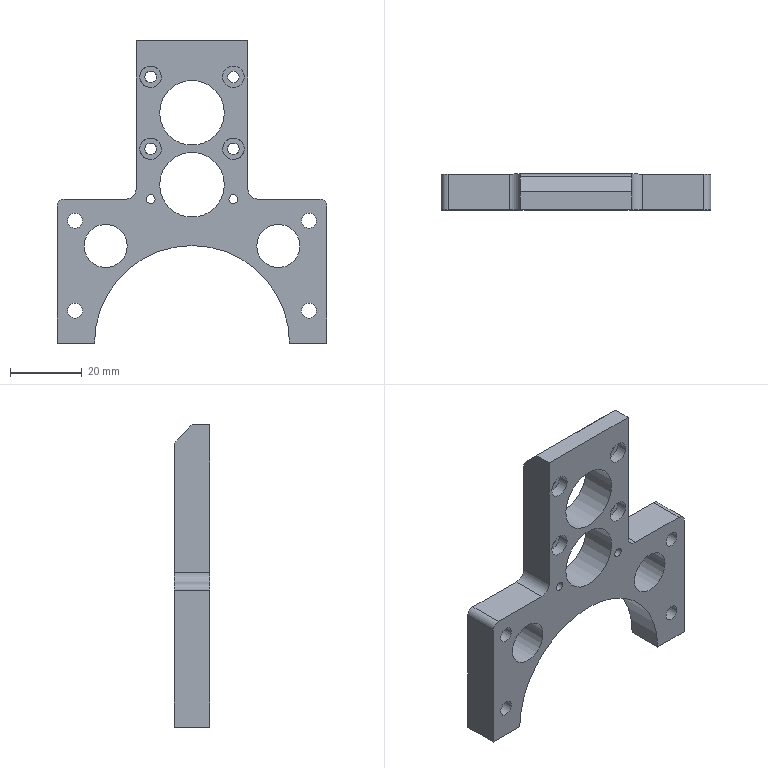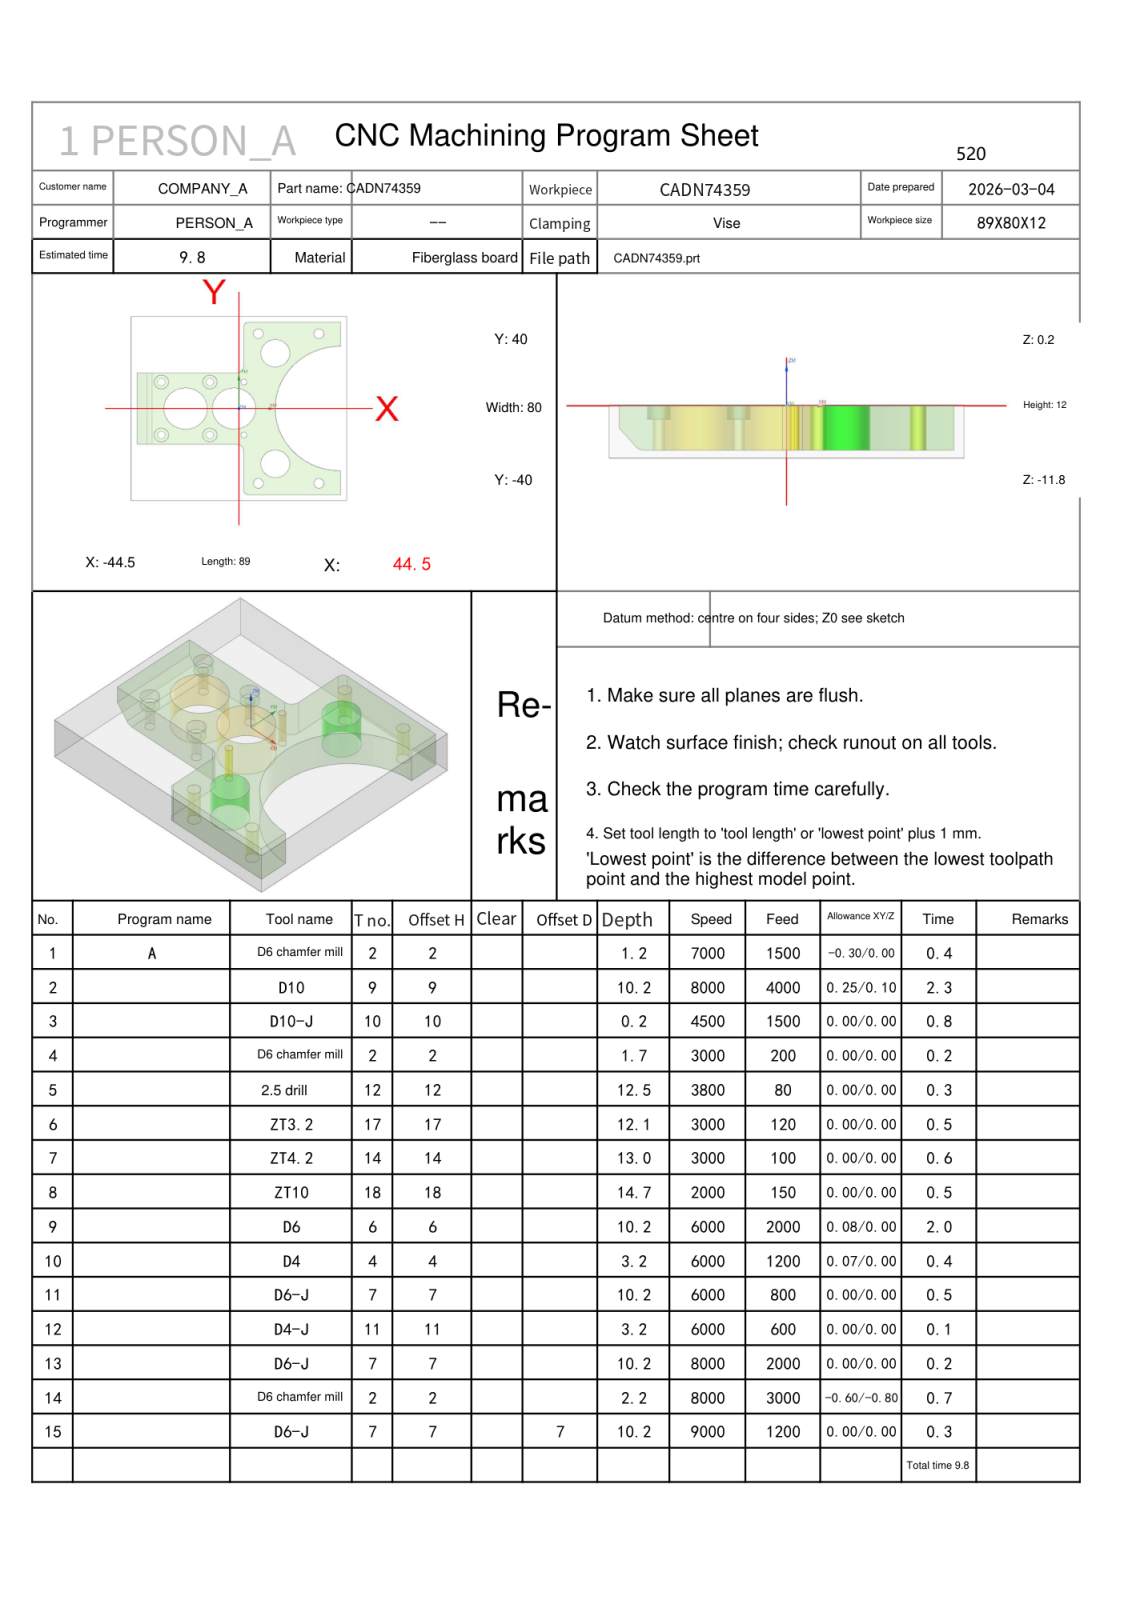NC program | NX | posted by the shop | part box 75 x 10 x 84 mm
Lines 1951 to 2989 of 4435:
N3 T10 M06
(D10-J  D=10. R=0. H=10 ce=0.00 di=0.00)
G00 G90 G54 X52. Y-35.962 M03 S4500
G43 H10 Z50.
M08
Z2.
G01 Z0.0 F1500.
X47.
X-47.
Y-29.423
X47.
Y-22.885
X-47.
Y-16.346
X47.
Y-9.808
X-47.
Y-3.269
X47.
Y3.269
X-47.
Y9.808
X47.
Y16.346
X-47.
Y22.885
X47.
Y29.423
X-47.
Y35.962
X47.
X52.
Z2.
G00 Z50.
G91 G28 Z0.0
M05
M09
G91 G28 Z0.0
M01
N4 T02 M06
(D6 chamfer mill  D=6. R=0. H=02 ce=0.00 di=0.00)
G00 G90 G54 X2. Y11.5 M03 S3000
G43 H02 Z50.
M08
G98 G81 X2. Y11.5 Z-1. R1. F200.
Y-11.5
G80
G00 Z50.
G00 G90 X33. Y-32.5 M03 S3000
Z50.
G98 G81 X33. Y-32.5 Z-1.5 R1. F200.
X15. Y-24.
X8. Y-32.5
X-12. Y-11.5
X-32.
X-22. Y0.0
X-32. Y11.5
X-12.
X-2. Y0.0
X8. Y32.5
X15. Y24.
X33. Y32.5
G80
G00 Z50.
G91 G28 Z0.0
M05
M09
G91 G28 Z0.0
M01
N5 T12 M06
(2.5 drill D=2.5 DR_a=118 H=12)
G00 G90 G54 X2. Y11.5 M03 S3800
G43 H12 Z50.
M08
G98 G83 X2. Y11.5 Z-12.251 R1. F80. Q1.5
Y-11.5
G80
G00 Z50.
G91 G28 Z0.0
M05
M09
G91 G28 Z0.0
M01
N6 T17 M06
(ZT3.2 D=3.2 DR_a=120 H=17)
G00 G90 G54 X-12. Y-11.5 M03 S3000
G43 H17 Z50.
M08
G98 G83 X-12. Y-11.5 Z-11.924 R1. F120. Q3.
X-32.
Y11.5
X-12.
G80
G00 Z50.
G91 G28 Z0.0
M05
M09
G91 G28 Z0.0
M01
N7 T14 M06
(ZT4.2 D=4.2 DR_a=118 H=14)
G00 G90 G54 X33. Y32.5 M03 S3000
G43 H14 Z50.
M08
G98 G83 X33. Y32.5 Z-12.762 R1. F100. Q1.5
X8.
Y-32.5
X33.
G80
G00 Z50.
G91 G28 Z0.0
M05
M09
G91 G28 Z0.0
M01
N8 T18 M06
(ZT10 D=10. DR_a=118 H=18)
G00 G90 G54 X15. Y-24. M03 S2000
G43 H18 Z50.
M08
G98 G83 X15. Y-24. Z-14.004 R1. F150. Q3.
Y24.
G80
G00 Z50.
G00 G90 X-22. Y0.0 M03 S2000
Z50.
G98 G83 X-22. Y0.0 Z-14.504 R1. F120. Q1.5
X-2.
G80
G00 Z50.
G91 G28 Z0.0
M05
M09
G91 G28 Z0.0
M01
N9 T06 M06
(D6  D=6. R=0. H=06 ce=0.10 di=0.00)
G00 G90 G54 X15. Y-24. M03 S6000
G43 H06 Z50.
M08
Z.3
G03 X16.45 Y-22.55 I0.0 J1.45 F2000.
X15. Y-21.1 I-1.45 J0.0
X15. Y-21.1 Z-.2 I0.0 J-2.9
X15. Y-21.1 Z-.7 I0.0 J-2.9
X15. Y-21.1 Z-1.2 I0.0 J-2.9
X15. Y-21.1 Z-1.7 I0.0 J-2.9
X15. Y-21.1 Z-2.2 I0.0 J-2.9
X15. Y-21.1 Z-2.7 I0.0 J-2.9
X15. Y-21.1 Z-3.2 I0.0 J-2.9
X15. Y-21.1 Z-3.7 I0.0 J-2.9
X15. Y-21.1 Z-4.2 I0.0 J-2.9
X15. Y-21.1 Z-4.7 I0.0 J-2.9
X15. Y-21.1 Z-5.2 I0.0 J-2.9
X15. Y-21.1 Z-5.7 I0.0 J-2.9
X15. Y-21.1 Z-6.2 I0.0 J-2.9
X15. Y-21.1 Z-6.7 I0.0 J-2.9
X15. Y-21.1 Z-7.2 I0.0 J-2.9
X15. Y-21.1 Z-7.7 I0.0 J-2.9
X15. Y-21.1 Z-8.2 I0.0 J-2.9
X15. Y-21.1 Z-8.7 I0.0 J-2.9
X15. Y-21.1 Z-9.2 I0.0 J-2.9
X15. Y-21.1 Z-9.7 I0.0 J-2.9
X16.705 Y-26.346 Z-10. I0.0 J-2.9
X17.9 Y-24. I-1.705 J2.346
X15. Y-21.1 I-2.9 J0.0
X12.1 Y-24. I0.0 J-2.9
X15. Y-26.9 I2.9 J0.0
X16.705 Y-26.346 I0.0 J2.9
X17.302 Y-25.173 I-.852 J1.173
X15.852 Y-23.723 I-1.45 J0.0
X15. Y-24. I0.0 J-1.45
G00 Z50.
Y24.
Z.3
G03 X16.45 Y25.45 I0.0 J1.45
X15. Y26.9 I-1.45 J0.0
X15. Y26.9 Z-.2 I0.0 J-2.9
X15. Y26.9 Z-.7 I0.0 J-2.9
X15. Y26.9 Z-1.2 I0.0 J-2.9
X15. Y26.9 Z-1.7 I0.0 J-2.9
X15. Y26.9 Z-2.2 I0.0 J-2.9
X15. Y26.9 Z-2.7 I0.0 J-2.9
X15. Y26.9 Z-3.2 I0.0 J-2.9
X15. Y26.9 Z-3.7 I0.0 J-2.9
X15. Y26.9 Z-4.2 I0.0 J-2.9
X15. Y26.9 Z-4.7 I0.0 J-2.9
X15. Y26.9 Z-5.2 I0.0 J-2.9
X15. Y26.9 Z-5.7 I0.0 J-2.9
X15. Y26.9 Z-6.2 I0.0 J-2.9
X15. Y26.9 Z-6.7 I0.0 J-2.9
X15. Y26.9 Z-7.2 I0.0 J-2.9
X15. Y26.9 Z-7.7 I0.0 J-2.9
X15. Y26.9 Z-8.2 I0.0 J-2.9
X15. Y26.9 Z-8.7 I0.0 J-2.9
X15. Y26.9 Z-9.2 I0.0 J-2.9
X15. Y26.9 Z-9.7 I0.0 J-2.9
X16.705 Y21.654 Z-10. I0.0 J-2.9
X17.9 Y24. I-1.705 J2.346
X15. Y26.9 I-2.9 J0.0
X12.1 Y24. I0.0 J-2.9
X15. Y21.1 I2.9 J0.0
X16.705 Y21.654 I0.0 J2.9
X17.302 Y22.827 I-.852 J1.173
X15.852 Y24.277 I-1.45 J0.0
X15. Y24. I0.0 J-1.45
G00 Z50.
G00 G90 X-22. Y0.0 M03 S6000
Z50.
Z.5
G03 X-20.75 Y1.25 I0.0 J1.25 F1800.
X-22. Y2.5 I-1.25 J0.0
X-22. Y2.5 Z.3 I0.0 J-2.5 F2000.
X-22. Y2.5 Z.1 I0.0 J-2.5
X-22. Y2.5 Z-.1 I0.0 J-2.5
X-22. Y2.5 Z-.3 I0.0 J-2.5
X-22. Y2.5 Z-.5 I0.0 J-2.5
X-22. Y2.5 Z-.7 I0.0 J-2.5
X-22. Y2.5 Z-.9 I0.0 J-2.5
X-22. Y2.5 Z-1.1 I0.0 J-2.5
X-22. Y2.5 Z-1.3 I0.0 J-2.5
X-22. Y2.5 Z-1.5 I0.0 J-2.5
X-22. Y2.5 Z-1.7 I0.0 J-2.5
X-22. Y2.5 Z-1.9 I0.0 J-2.5
X-22. Y2.5 Z-2.1 I0.0 J-2.5
X-22. Y2.5 Z-2.3 I0.0 J-2.5
X-22. Y2.5 Z-2.5 I0.0 J-2.5
X-22. Y2.5 Z-2.7 I0.0 J-2.5
X-22. Y2.5 Z-2.9 I0.0 J-2.5
X-22. Y2.5 Z-3.1 I0.0 J-2.5
X-22. Y2.5 Z-3.3 I0.0 J-2.5
X-22. Y2.5 Z-3.5 I0.0 J-2.5
X-22. Y2.5 Z-3.7 I0.0 J-2.5
X-22. Y2.5 Z-3.9 I0.0 J-2.5
X-22. Y2.5 Z-4.1 I0.0 J-2.5
X-22. Y2.5 Z-4.3 I0.0 J-2.5
X-22. Y2.5 Z-4.5 I0.0 J-2.5
X-22. Y2.5 Z-4.7 I0.0 J-2.5
X-24.5 Y0.0 Z-4.75 I0.0 J-2.5
X-21.984 Y-2.552 I2.552 J0.0
G01 X-21.947
G03 X-19.352 Y-.072 I0.0 J2.598
G01 X-19.35 Y.049
G03 X-21.868 Y2.72 I-2.675 J0.0
G01 X-22.03 Y2.724
G03 X-24.793 Y.153 I0.0 J-2.77
X-24.8 Y-.05 I2.817 J-.202
X-22.216 Y-2.863 I2.824 J0.0
X-21.968 Y-2.874 I.248 J2.908
X-19.064 Y-.241 I0.0 J2.919
X-19.049 Y.05 I-2.958 J.291
X-21.692 Y3.004 I-2.973 J0.0
X-22.033 Y3.023 I-.341 J-3.048
X-25.076 Y.338 I0.0 J-3.067
X-25.101 Y-.051 I3.097 J-.388
X-22.409 Y-3.142 I3.121 J0.0
X-21.966 Y-3.173 I.442 J3.186
X-18.787 Y-.442 I0.0 J3.216
X-18.749 Y.051 I-3.233 J.493
X-21.483 Y3.277 I-3.27 J0.0
X-22.035 Y3.323 I-.552 J-3.319
X-25.347 Y.554 I0.0 J-3.365
X-25.401 Y-.052 I3.365 J-.605
X-22.632 Y-3.408 I3.419 J0.0
X-21.964 Y-3.472 I.668 J3.449
X-18.524 Y-.673 I0.0 J3.514
X-18.449 Y.052 I-3.493 J.725
X-21.245 Y3.535 I-3.568 J0.0
X-22.037 Y3.622 I-.792 J-3.576
X-25.602 Y.8 I0.0 J-3.662
X-25.701 Y-.053 I3.617 J-.853
X-22.886 Y-3.658 I3.716 J0.0
X-21.962 Y-3.772 I.924 J3.697
X-18.277 Y-.934 I0.0 J3.811
X-18.149 Y.053 I-3.737 J.987
X-20.977 Y3.776 I-3.865 J0.0
X-22.039 Y3.921 I-1.063 J-3.814
X-25.839 Y1.076 I0.0 J-3.96
X-26.001 Y-.053 I3.852 J-1.129
X-23.168 Y-3.889 I4.014 J0.0
X-21.96 Y-4.071 I1.209 J3.927
X-18.05 Y-1.224 I0.0 J4.108
X-17.849 Y.054 I-3.961 J1.278
X-20.68 Y3.998 I-4.162 J0.0
X-22.041 Y4.221 I-1.361 J-4.034
X-26.056 Y1.379 I0.0 J-4.257
X-26.301 Y-.054 I4.066 J-1.433
X-23.479 Y-4.1 I4.311 J0.0
X-21.958 Y-4.371 I1.521 J4.135
X-17.844 Y-1.541 I0.0 J4.406
X-17.548 Y.054 I-4.165 J1.596
X-20.356 Y4.197 I-4.46 J0.0
X-22.043 Y4.521 I-1.687 J-4.231
X-26.251 Y1.71 I0.0 J-4.555
X-26.602 Y-.054 I4.257 J-1.764
X-23.815 Y-4.288 I4.608 J0.0
X-21.956 Y-4.671 I1.859 J4.32
X-17.661 Y-1.885 I0.0 J4.703
X-17.248 Y.055 I-4.344 J1.939
X-20.007 Y4.372 I-4.757 J0.0
X-22.045 Y4.821 I-2.037 J-4.403
X-26.42 Y2.065 I0.0 J-4.852
X-26.902 Y-.055 I4.424 J-2.12
X-24.176 Y-4.45 I4.906 J0.0
X-21.954 Y-4.97 I2.222 J4.48
X-17.505 Y-2.252 I0.0 J5.001
X-16.948 Y.055 I-4.498 J2.307
X-19.635 Y4.521 I-5.055 J0.0
X-22.047 Y5.12 I-2.412 J-4.55
X-26.563 Y2.444 I0.0 J-5.149
X-27.203 Y-.055 I4.564 J-2.499
X-24.56 Y-4.585 I5.203 J0.0
X-21.953 Y-5.27 I2.607 J4.612
X-17.376 Y-2.642 I0.0 J5.298
X-16.647 Y.055 I-4.623 J2.696
X-19.24 Y4.641 I-5.352 J0.0
X-22.048 Y5.42 I-2.808 J-4.667
X-26.677 Y2.844 I0.0 J-5.447
X-27.503 Y-.055 I4.675 J-2.899
X-24.964 Y-4.69 I5.501 J0.0
X-21.951 Y-5.57 I3.013 J4.715
X-17.278 Y-3.052 I0.0 J5.595
X-16.347 Y.055 I-4.719 J3.106
X-18.826 Y4.731 I-5.649 J0.0
X-22.049 Y5.72 I-3.223 J-4.755
X-26.76 Y3.263 I0.0 J-5.744
X-27.808 Y-.068 I4.774 J-3.332
X-25.344 Y-4.824 I5.822 J0.0
X-21.959 Y-5.899 I3.385 J4.794
X-17.211 Y-3.48 I0.0 J5.869
X-16.08 Y0.0 I-4.789 J3.48
X-22. Y5.92 I-5.92 J0.0
X-27.92 Y0.0 I0.0 J-5.92
X-22. Y-5.92 I5.92 J0.0
X-16.934 Y-3.063 I0.0 J5.92
X-16.507 Y-1.532 I-2.533 J1.532
X-19.467 Y1.428 I-2.96 J0.0
X-22. Y0.0 I0.0 J-2.96
X-20.75 Y1.25 I0.0 J1.25 F1800.
X-22. Y2.5 I-1.25 J0.0
X-22. Y2.5 Z-4.95 I0.0 J-2.5 F2000.
X-22. Y2.5 Z-5.15 I0.0 J-2.5
X-22. Y2.5 Z-5.35 I0.0 J-2.5
X-22. Y2.5 Z-5.55 I0.0 J-2.5
X-22. Y2.5 Z-5.75 I0.0 J-2.5
X-22. Y2.5 Z-5.95 I0.0 J-2.5
X-22. Y2.5 Z-6.15 I0.0 J-2.5
X-22. Y2.5 Z-6.35 I0.0 J-2.5
X-22. Y2.5 Z-6.55 I0.0 J-2.5
X-22. Y2.5 Z-6.75 I0.0 J-2.5
X-22. Y2.5 Z-6.95 I0.0 J-2.5
X-22. Y2.5 Z-7.15 I0.0 J-2.5
X-22. Y2.5 Z-7.35 I0.0 J-2.5
X-22. Y2.5 Z-7.55 I0.0 J-2.5
X-22. Y2.5 Z-7.75 I0.0 J-2.5
X-22. Y2.5 Z-7.95 I0.0 J-2.5
X-22. Y2.5 Z-8.15 I0.0 J-2.5
X-22. Y2.5 Z-8.35 I0.0 J-2.5
X-22. Y2.5 Z-8.55 I0.0 J-2.5
X-22. Y2.5 Z-8.75 I0.0 J-2.5
X-22. Y2.5 Z-8.95 I0.0 J-2.5
X-22. Y2.5 Z-9.15 I0.0 J-2.5
X-22. Y2.5 Z-9.35 I0.0 J-2.5
X-22. Y2.5 Z-9.55 I0.0 J-2.5
X-22. Y2.5 Z-9.75 I0.0 J-2.5
X-22. Y2.5 Z-9.95 I0.0 J-2.5
X-24.5 Y0.0 Z-10. I0.0 J-2.5
X-21.984 Y-2.552 I2.552 J0.0
G01 X-21.947
G03 X-19.352 Y-.072 I0.0 J2.598
G01 X-19.35 Y.049
G03 X-21.868 Y2.72 I-2.675 J0.0
G01 X-22.03 Y2.724
G03 X-24.793 Y.153 I0.0 J-2.77
X-24.8 Y-.05 I2.817 J-.202
X-22.216 Y-2.863 I2.824 J0.0
X-21.968 Y-2.874 I.248 J2.908
X-19.064 Y-.241 I0.0 J2.919
X-19.049 Y.05 I-2.958 J.291
X-21.692 Y3.004 I-2.973 J0.0
X-22.033 Y3.023 I-.341 J-3.048
X-25.076 Y.338 I0.0 J-3.067
X-25.101 Y-.051 I3.097 J-.388
X-22.409 Y-3.142 I3.121 J0.0
X-21.966 Y-3.173 I.442 J3.186
X-18.787 Y-.442 I0.0 J3.216
X-18.749 Y.051 I-3.233 J.493
X-21.483 Y3.277 I-3.27 J0.0
X-22.035 Y3.323 I-.552 J-3.319
X-25.347 Y.554 I0.0 J-3.365
X-25.401 Y-.052 I3.365 J-.605
X-22.632 Y-3.408 I3.419 J0.0
X-21.964 Y-3.472 I.668 J3.449
X-18.524 Y-.673 I0.0 J3.514
X-18.449 Y.052 I-3.493 J.725
X-21.245 Y3.535 I-3.568 J0.0
X-22.037 Y3.622 I-.792 J-3.576
X-25.602 Y.8 I0.0 J-3.662
X-25.701 Y-.053 I3.617 J-.853
X-22.886 Y-3.658 I3.716 J0.0
X-21.962 Y-3.772 I.924 J3.697
X-18.277 Y-.934 I0.0 J3.811
X-18.149 Y.053 I-3.737 J.987
X-20.977 Y3.776 I-3.865 J0.0
X-22.039 Y3.921 I-1.063 J-3.814
X-25.839 Y1.076 I0.0 J-3.96
X-26.001 Y-.053 I3.852 J-1.129
X-23.168 Y-3.889 I4.014 J0.0
X-21.96 Y-4.071 I1.209 J3.927
X-18.05 Y-1.224 I0.0 J4.108
X-17.849 Y.054 I-3.961 J1.278
X-20.68 Y3.998 I-4.162 J0.0
X-22.041 Y4.221 I-1.361 J-4.034
X-26.056 Y1.379 I0.0 J-4.257
X-26.301 Y-.054 I4.066 J-1.433
X-23.479 Y-4.1 I4.311 J0.0
X-21.958 Y-4.371 I1.521 J4.135
X-17.844 Y-1.541 I0.0 J4.406
X-17.548 Y.054 I-4.165 J1.596
X-20.356 Y4.197 I-4.46 J0.0
X-22.043 Y4.521 I-1.687 J-4.231
X-26.251 Y1.71 I0.0 J-4.555
X-26.602 Y-.054 I4.257 J-1.764
X-23.815 Y-4.288 I4.608 J0.0
X-21.956 Y-4.671 I1.859 J4.32
X-17.661 Y-1.885 I0.0 J4.703
X-17.248 Y.055 I-4.344 J1.939
X-20.007 Y4.372 I-4.757 J0.0
X-22.045 Y4.821 I-2.037 J-4.403
X-26.42 Y2.065 I0.0 J-4.852
X-26.902 Y-.055 I4.424 J-2.12
X-24.176 Y-4.45 I4.906 J0.0
X-21.954 Y-4.97 I2.222 J4.48
X-17.505 Y-2.252 I0.0 J5.001
X-16.948 Y.055 I-4.498 J2.307
X-19.635 Y4.521 I-5.055 J0.0
X-22.047 Y5.12 I-2.412 J-4.55
X-26.563 Y2.444 I0.0 J-5.149
X-27.203 Y-.055 I4.564 J-2.499
X-24.56 Y-4.585 I5.203 J0.0
X-21.953 Y-5.27 I2.607 J4.612
X-17.376 Y-2.642 I0.0 J5.298
X-16.647 Y.055 I-4.623 J2.696
X-19.24 Y4.641 I-5.352 J0.0
X-22.048 Y5.42 I-2.808 J-4.667
X-26.677 Y2.844 I0.0 J-5.447
X-27.503 Y-.055 I4.675 J-2.899
X-24.964 Y-4.69 I5.501 J0.0
X-21.951 Y-5.57 I3.013 J4.715
X-17.278 Y-3.052 I0.0 J5.595
X-16.347 Y.055 I-4.719 J3.106
X-18.826 Y4.731 I-5.649 J0.0
X-22.049 Y5.72 I-3.223 J-4.755
X-26.76 Y3.263 I0.0 J-5.744
X-27.808 Y-.068 I4.774 J-3.332
X-25.344 Y-4.824 I5.822 J0.0
X-21.959 Y-5.899 I3.385 J4.794
X-17.211 Y-3.48 I0.0 J5.869
X-16.08 Y0.0 I-4.789 J3.48
X-22. Y5.92 I-5.92 J0.0
X-27.92 Y0.0 I0.0 J-5.92
X-22. Y-5.92 I5.92 J0.0
X-16.934 Y-3.063 I0.0 J5.92
X-16.507 Y-1.532 I-2.533 J1.532
X-19.467 Y1.428 I-2.96 J0.0
X-22. Y0.0 I0.0 J-2.96
G00 Z50.
X-2.
Z.5
G03 X-.75 Y1.25 I0.0 J1.25 F1800.
X-2. Y2.5 I-1.25 J0.0
X-2. Y2.5 Z.3 I0.0 J-2.5 F2000.
X-2. Y2.5 Z.1 I0.0 J-2.5
X-2. Y2.5 Z-.1 I0.0 J-2.5
X-2. Y2.5 Z-.3 I0.0 J-2.5
X-2. Y2.5 Z-.5 I0.0 J-2.5
X-2. Y2.5 Z-.7 I0.0 J-2.5
X-2. Y2.5 Z-.9 I0.0 J-2.5
X-2. Y2.5 Z-1.1 I0.0 J-2.5
X-2. Y2.5 Z-1.3 I0.0 J-2.5
X-2. Y2.5 Z-1.5 I0.0 J-2.5
X-2. Y2.5 Z-1.7 I0.0 J-2.5
X-2. Y2.5 Z-1.9 I0.0 J-2.5
X-2. Y2.5 Z-2.1 I0.0 J-2.5
X-2. Y2.5 Z-2.3 I0.0 J-2.5
X-2. Y2.5 Z-2.5 I0.0 J-2.5
X-2. Y2.5 Z-2.7 I0.0 J-2.5
X-2. Y2.5 Z-2.9 I0.0 J-2.5
X-2. Y2.5 Z-3.1 I0.0 J-2.5
X-2. Y2.5 Z-3.3 I0.0 J-2.5
X-2. Y2.5 Z-3.5 I0.0 J-2.5
X-2. Y2.5 Z-3.7 I0.0 J-2.5
X-2. Y2.5 Z-3.9 I0.0 J-2.5
X-2. Y2.5 Z-4.1 I0.0 J-2.5
X-2. Y2.5 Z-4.3 I0.0 J-2.5
X-2. Y2.5 Z-4.5 I0.0 J-2.5
X-2. Y2.5 Z-4.7 I0.0 J-2.5
X-4.5 Y0.0 Z-4.75 I0.0 J-2.5
X-1.984 Y-2.552 I2.552 J0.0
G01 X-1.947
G03 X.648 Y-.072 I0.0 J2.598
G01 X.65 Y.049
G03 X-1.868 Y2.72 I-2.675 J0.0
G01 X-2.03 Y2.724
G03 X-4.793 Y.153 I0.0 J-2.77
X-4.8 Y-.05 I2.817 J-.202
X-2.216 Y-2.863 I2.824 J0.0
X-1.968 Y-2.874 I.248 J2.908
X.936 Y-.241 I0.0 J2.919
X.951 Y.05 I-2.958 J.291
X-1.692 Y3.004 I-2.973 J0.0
X-2.033 Y3.023 I-.341 J-3.048
X-5.076 Y.338 I0.0 J-3.067
X-5.101 Y-.051 I3.097 J-.388
X-2.409 Y-3.142 I3.121 J0.0
X-1.966 Y-3.173 I.442 J3.186
X1.213 Y-.442 I0.0 J3.216
X1.251 Y.051 I-3.233 J.493
X-1.483 Y3.277 I-3.27 J0.0
X-2.035 Y3.323 I-.552 J-3.319
X-5.347 Y.554 I0.0 J-3.365
X-5.401 Y-.052 I3.365 J-.605
X-2.632 Y-3.408 I3.419 J0.0
X-1.964 Y-3.472 I.668 J3.449
X1.476 Y-.673 I0.0 J3.514
X1.551 Y.052 I-3.493 J.725
X-1.245 Y3.535 I-3.568 J0.0
X-2.037 Y3.622 I-.792 J-3.576
X-5.602 Y.8 I0.0 J-3.662
X-5.701 Y-.053 I3.617 J-.853
X-2.886 Y-3.658 I3.716 J0.0
X-1.962 Y-3.772 I.924 J3.697
X1.723 Y-.934 I0.0 J3.811
X1.851 Y.053 I-3.737 J.987
X-.977 Y3.776 I-3.865 J0.0
X-2.039 Y3.921 I-1.063 J-3.814
X-5.839 Y1.076 I0.0 J-3.96
X-6.001 Y-.053 I3.852 J-1.129
X-3.168 Y-3.889 I4.014 J0.0
X-1.96 Y-4.071 I1.209 J3.927
X1.95 Y-1.224 I0.0 J4.108
X2.151 Y.054 I-3.961 J1.278
X-.68 Y3.998 I-4.162 J0.0
X-2.041 Y4.221 I-1.361 J-4.034
X-6.056 Y1.379 I0.0 J-4.257
X-6.301 Y-.054 I4.066 J-1.433
X-3.479 Y-4.1 I4.311 J0.0
X-1.958 Y-4.371 I1.521 J4.135
X2.156 Y-1.541 I0.0 J4.406
X2.452 Y.054 I-4.165 J1.596
X-.356 Y4.197 I-4.46 J0.0
X-2.043 Y4.521 I-1.687 J-4.231
X-6.251 Y1.71 I0.0 J-4.555
X-6.602 Y-.054 I4.257 J-1.764
X-3.815 Y-4.288 I4.608 J0.0
X-1.956 Y-4.671 I1.859 J4.32
X2.339 Y-1.885 I0.0 J4.703
X2.752 Y.055 I-4.344 J1.939
X-.007 Y4.372 I-4.757 J0.0
X-2.045 Y4.821 I-2.037 J-4.403
X-6.42 Y2.065 I0.0 J-4.852
X-6.902 Y-.055 I4.424 J-2.12
X-4.176 Y-4.45 I4.906 J0.0
X-1.954 Y-4.97 I2.222 J4.48
X2.495 Y-2.252 I0.0 J5.001
X3.052 Y.055 I-4.498 J2.307
X.365 Y4.521 I-5.055 J0.0
X-2.047 Y5.12 I-2.412 J-4.55
X-6.563 Y2.444 I0.0 J-5.149
X-7.203 Y-.055 I4.564 J-2.499
X-4.56 Y-4.585 I5.203 J0.0
X-1.953 Y-5.27 I2.607 J4.612
X2.624 Y-2.642 I0.0 J5.298
X3.353 Y.055 I-4.623 J2.696
X.76 Y4.641 I-5.352 J0.0
X-2.048 Y5.42 I-2.808 J-4.667
X-6.677 Y2.844 I0.0 J-5.447
X-7.503 Y-.055 I4.675 J-2.899
X-4.964 Y-4.69 I5.501 J0.0
X-1.951 Y-5.57 I3.013 J4.715
X2.722 Y-3.052 I0.0 J5.595
X3.653 Y.055 I-4.719 J3.106
X1.174 Y4.731 I-5.649 J0.0
X-2.049 Y5.72 I-3.223 J-4.755
X-6.76 Y3.263 I0.0 J-5.744
X-7.808 Y-.068 I4.774 J-3.332
X-5.344 Y-4.824 I5.822 J0.0
X-1.959 Y-5.899 I3.385 J4.794
X2.789 Y-3.48 I0.0 J5.869
X3.92 Y0.0 I-4.789 J3.48
X-2. Y5.92 I-5.92 J0.0
X-7.92 Y0.0 I0.0 J-5.92
X-2. Y-5.92 I5.92 J0.0
X3.066 Y-3.063 I0.0 J5.92
X3.493 Y-1.532 I-2.533 J1.532
X.533 Y1.428 I-2.96 J0.0
X-2. Y0.0 I0.0 J-2.96
X-.75 Y1.25 I0.0 J1.25 F1800.
X-2. Y2.5 I-1.25 J0.0
X-2. Y2.5 Z-4.95 I0.0 J-2.5 F2000.
X-2. Y2.5 Z-5.15 I0.0 J-2.5
X-2. Y2.5 Z-5.35 I0.0 J-2.5
X-2. Y2.5 Z-5.55 I0.0 J-2.5
X-2. Y2.5 Z-5.75 I0.0 J-2.5
X-2. Y2.5 Z-5.95 I0.0 J-2.5
X-2. Y2.5 Z-6.15 I0.0 J-2.5
X-2. Y2.5 Z-6.35 I0.0 J-2.5
X-2. Y2.5 Z-6.55 I0.0 J-2.5
X-2. Y2.5 Z-6.75 I0.0 J-2.5
X-2. Y2.5 Z-6.95 I0.0 J-2.5
X-2. Y2.5 Z-7.15 I0.0 J-2.5
X-2. Y2.5 Z-7.35 I0.0 J-2.5
X-2. Y2.5 Z-7.55 I0.0 J-2.5
X-2. Y2.5 Z-7.75 I0.0 J-2.5
X-2. Y2.5 Z-7.95 I0.0 J-2.5
X-2. Y2.5 Z-8.15 I0.0 J-2.5
X-2. Y2.5 Z-8.35 I0.0 J-2.5
X-2. Y2.5 Z-8.55 I0.0 J-2.5
X-2. Y2.5 Z-8.75 I0.0 J-2.5
X-2. Y2.5 Z-8.95 I0.0 J-2.5
X-2. Y2.5 Z-9.15 I0.0 J-2.5
X-2. Y2.5 Z-9.35 I0.0 J-2.5
X-2. Y2.5 Z-9.55 I0.0 J-2.5
X-2. Y2.5 Z-9.75 I0.0 J-2.5
X-2. Y2.5 Z-9.95 I0.0 J-2.5
X-4.5 Y0.0 Z-10. I0.0 J-2.5
X-1.984 Y-2.552 I2.552 J0.0
G01 X-1.947
G03 X.648 Y-.072 I0.0 J2.598
G01 X.65 Y.049
G03 X-1.868 Y2.72 I-2.675 J0.0
G01 X-2.03 Y2.724
G03 X-4.793 Y.153 I0.0 J-2.77
X-4.8 Y-.05 I2.817 J-.202
X-2.216 Y-2.863 I2.824 J0.0
X-1.968 Y-2.874 I.248 J2.908
X.936 Y-.241 I0.0 J2.919
X.951 Y.05 I-2.958 J.291
X-1.692 Y3.004 I-2.973 J0.0
X-2.033 Y3.023 I-.341 J-3.048
X-5.076 Y.338 I0.0 J-3.067
X-5.101 Y-.051 I3.097 J-.388
X-2.409 Y-3.142 I3.121 J0.0
X-1.966 Y-3.173 I.442 J3.186
X1.213 Y-.442 I0.0 J3.216
X1.251 Y.051 I-3.233 J.493
X-1.483 Y3.277 I-3.27 J0.0
X-2.035 Y3.323 I-.552 J-3.319
X-5.347 Y.554 I0.0 J-3.365
X-5.401 Y-.052 I3.365 J-.605
X-2.632 Y-3.408 I3.419 J0.0
X-1.964 Y-3.472 I.668 J3.449
X1.476 Y-.673 I0.0 J3.514
X1.551 Y.052 I-3.493 J.725
X-1.245 Y3.535 I-3.568 J0.0
X-2.037 Y3.622 I-.792 J-3.576
X-5.602 Y.8 I0.0 J-3.662
X-5.701 Y-.053 I3.617 J-.853
X-2.886 Y-3.658 I3.716 J0.0
X-1.962 Y-3.772 I.924 J3.697
X1.723 Y-.934 I0.0 J3.811
X1.851 Y.053 I-3.737 J.987
X-.977 Y3.776 I-3.865 J0.0
X-2.039 Y3.921 I-1.063 J-3.814
X-5.839 Y1.076 I0.0 J-3.96
X-6.001 Y-.053 I3.852 J-1.129
X-3.168 Y-3.889 I4.014 J0.0
X-1.96 Y-4.071 I1.209 J3.927
X1.95 Y-1.224 I0.0 J4.108
X2.151 Y.054 I-3.961 J1.278
X-.68 Y3.998 I-4.162 J0.0
X-2.041 Y4.221 I-1.361 J-4.034
X-6.056 Y1.379 I0.0 J-4.257
X-6.301 Y-.054 I4.066 J-1.433
X-3.479 Y-4.1 I4.311 J0.0
X-1.958 Y-4.371 I1.521 J4.135
X2.156 Y-1.541 I0.0 J4.406
X2.452 Y.054 I-4.165 J1.596
X-.356 Y4.197 I-4.46 J0.0
X-2.043 Y4.521 I-1.687 J-4.231
X-6.251 Y1.71 I0.0 J-4.555
X-6.602 Y-.054 I4.257 J-1.764
X-3.815 Y-4.288 I4.608 J0.0
X-1.956 Y-4.671 I1.859 J4.32
X2.339 Y-1.885 I0.0 J4.703
X2.752 Y.055 I-4.344 J1.939
X-.007 Y4.372 I-4.757 J0.0
X-2.045 Y4.821 I-2.037 J-4.403
X-6.42 Y2.065 I0.0 J-4.852
X-6.902 Y-.055 I4.424 J-2.12
X-4.176 Y-4.45 I4.906 J0.0
X-1.954 Y-4.97 I2.222 J4.48
X2.495 Y-2.252 I0.0 J5.001
X3.052 Y.055 I-4.498 J2.307
X.365 Y4.521 I-5.055 J0.0
X-2.047 Y5.12 I-2.412 J-4.55
X-6.563 Y2.444 I0.0 J-5.149
X-7.203 Y-.055 I4.564 J-2.499
X-4.56 Y-4.585 I5.203 J0.0
X-1.953 Y-5.27 I2.607 J4.612
X2.624 Y-2.642 I0.0 J5.298
X3.353 Y.055 I-4.623 J2.696
X.76 Y4.641 I-5.352 J0.0
X-2.048 Y5.42 I-2.808 J-4.667
X-6.677 Y2.844 I0.0 J-5.447
X-7.503 Y-.055 I4.675 J-2.899
X-4.964 Y-4.69 I5.501 J0.0
X-1.951 Y-5.57 I3.013 J4.715
X2.722 Y-3.052 I0.0 J5.595
X3.653 Y.055 I-4.719 J3.106
X1.174 Y4.731 I-5.649 J0.0
X-2.049 Y5.72 I-3.223 J-4.755
X-6.76 Y3.263 I0.0 J-5.744
X-7.808 Y-.068 I4.774 J-3.332
X-5.344 Y-4.824 I5.822 J0.0
X-1.959 Y-5.899 I3.385 J4.794
X2.789 Y-3.48 I0.0 J5.869
X3.92 Y0.0 I-4.789 J3.48
X-2. Y5.92 I-5.92 J0.0
X-7.92 Y0.0 I0.0 J-5.92
X-2. Y-5.92 I5.92 J0.0
X3.066 Y-3.063 I0.0 J5.92
X3.493 Y-1.532 I-2.533 J1.532
X.533 Y1.428 I-2.96 J0.0
X-2. Y0.0 I0.0 J-2.96
G00 Z50.
G91 G28 Z0.0
M05
M09
G91 G28 Z0.0
M01
N10 T04 M06
(D4  D=4. R=0. H=04 ce=0.07 di=0.00)
G00 G90 G54 X-12. Y-11.5 M03 S6000
G43 H04 Z50.
M08
Z.3
G03 X-11.535 Y-11.035 I0.0 J.465 F1200.
X-12. Y-10.57 I-.465 J0.0
X-12. Y-10.57 Z.1 I0.0 J-.93
X-12. Y-10.57 Z-.1 I0.0 J-.93
X-12. Y-10.57 Z-.3 I0.0 J-.93
X-12. Y-10.57 Z-.5 I0.0 J-.93
X-12. Y-10.57 Z-.7 I0.0 J-.93
X-12. Y-10.57 Z-.9 I0.0 J-.93
X-12. Y-10.57 Z-1.1 I0.0 J-.93
X-12. Y-10.57 Z-1.3 I0.0 J-.93
X-12. Y-10.57 Z-1.5 I0.0 J-.93
X-12. Y-10.57 Z-1.7 I0.0 J-.93
X-12. Y-10.57 Z-1.9 I0.0 J-.93
X-12. Y-10.57 Z-2.1 I0.0 J-.93
X-12. Y-10.57 Z-2.3 I0.0 J-.93
X-12. Y-10.57 Z-2.5 I0.0 J-.93
X-12. Y-10.57 Z-2.7 I0.0 J-.93
X-12. Y-10.57 Z-2.9 I0.0 J-.93
X-12. Y-12.43 Z-3. I0.0 J-.93
X-11.07 Y-11.5 I0.0 J.93
X-12. Y-10.57 I-.93 J0.0
X-12.93 Y-11.5 I0.0 J-.93
X-12. Y-12.43 I.93 J0.0
X-11.535 Y-11.965 I0.0 J.465
X-12. Y-11.5 I-.465 J0.0
G00 Z50.
X-32.
Z.3
G03 X-31.535 Y-11.035 I0.0 J.465
X-32. Y-10.57 I-.465 J0.0
X-32. Y-10.57 Z.1 I0.0 J-.93
X-32. Y-10.57 Z-.1 I0.0 J-.93
X-32. Y-10.57 Z-.3 I0.0 J-.93
X-32. Y-10.57 Z-.5 I0.0 J-.93
X-32. Y-10.57 Z-.7 I0.0 J-.93
X-32. Y-10.57 Z-.9 I0.0 J-.93
X-32. Y-10.57 Z-1.1 I0.0 J-.93
X-32. Y-10.57 Z-1.3 I0.0 J-.93
X-32. Y-10.57 Z-1.5 I0.0 J-.93
X-32. Y-10.57 Z-1.7 I0.0 J-.93
X-32. Y-10.57 Z-1.9 I0.0 J-.93
X-32. Y-10.57 Z-2.1 I0.0 J-.93
X-32. Y-10.57 Z-2.3 I0.0 J-.93
X-32. Y-10.57 Z-2.5 I0.0 J-.93
X-32. Y-10.57 Z-2.7 I0.0 J-.93
X-32. Y-10.57 Z-2.9 I0.0 J-.93
X-32. Y-12.43 Z-3. I0.0 J-.93
X-31.07 Y-11.5 I0.0 J.93
X-32. Y-10.57 I-.93 J0.0
X-32.93 Y-11.5 I0.0 J-.93
X-32. Y-12.43 I.93 J0.0
X-31.535 Y-11.965 I0.0 J.465
X-32. Y-11.5 I-.465 J0.0
G00 Z50.
G00 G90 X-12. Y11.5 M03 S6000
Z50.
Z.3
G03 X-11.535 Y11.965 I0.0 J.465 F1200.
X-12. Y12.43 I-.465 J0.0
X-12. Y12.43 Z.1 I0.0 J-.93
X-12. Y12.43 Z-.1 I0.0 J-.93
X-12. Y12.43 Z-.3 I0.0 J-.93
X-12. Y12.43 Z-.5 I0.0 J-.93
X-12. Y12.43 Z-.7 I0.0 J-.93
X-12. Y12.43 Z-.9 I0.0 J-.93
X-12. Y12.43 Z-1.1 I0.0 J-.93
X-12. Y12.43 Z-1.3 I0.0 J-.93
X-12. Y12.43 Z-1.5 I0.0 J-.93
X-12. Y12.43 Z-1.7 I0.0 J-.93
X-12. Y12.43 Z-1.9 I0.0 J-.93
X-12. Y12.43 Z-2.1 I0.0 J-.93
X-12. Y12.43 Z-2.3 I0.0 J-.93
X-12. Y12.43 Z-2.5 I0.0 J-.93
X-12. Y12.43 Z-2.7 I0.0 J-.93
X-12. Y12.43 Z-2.9 I0.0 J-.93
X-12. Y10.57 Z-3. I0.0 J-.93
X-11.07 Y11.5 I0.0 J.93
X-12. Y12.43 I-.93 J0.0
X-12.93 Y11.5 I0.0 J-.93
X-12. Y10.57 I.93 J0.0
X-11.535 Y11.035 I0.0 J.465
X-12. Y11.5 I-.465 J0.0
G00 Z50.
X-32.
Z.3
G03 X-31.535 Y11.965 I0.0 J.465
X-32. Y12.43 I-.465 J0.0
X-32. Y12.43 Z.1 I0.0 J-.93
X-32. Y12.43 Z-.1 I0.0 J-.93
X-32. Y12.43 Z-.3 I0.0 J-.93
X-32. Y12.43 Z-.5 I0.0 J-.93
X-32. Y12.43 Z-.7 I0.0 J-.93
X-32. Y12.43 Z-.9 I0.0 J-.93
X-32. Y12.43 Z-1.1 I0.0 J-.93
X-32. Y12.43 Z-1.3 I0.0 J-.93
X-32. Y12.43 Z-1.5 I0.0 J-.93
X-32. Y12.43 Z-1.7 I0.0 J-.93
X-32. Y12.43 Z-1.9 I0.0 J-.93
X-32. Y12.43 Z-2.1 I0.0 J-.93
X-32. Y12.43 Z-2.3 I0.0 J-.93
X-32. Y12.43 Z-2.5 I0.0 J-.93
X-32. Y12.43 Z-2.7 I0.0 J-.93
X-32. Y12.43 Z-2.9 I0.0 J-.93
X-32. Y10.57 Z-3. I0.0 J-.93
X-31.07 Y11.5 I0.0 J.93
X-32. Y12.43 I-.93 J0.0
X-32.93 Y11.5 I0.0 J-.93
X-32. Y10.57 I.93 J0.0
X-31.535 Y11.035 I0.0 J.465
X-32. Y11.5 I-.465 J0.0
G00 Z50.
G91 G28 Z0.0
M05
M09
G91 G28 Z0.0
M01
N11 T07 M06
(D6-J  D=6. R=0. H=07 ce=0.00 di=0.00)
G00 G90 G54 X15. Y-24. M03 S6000
G43 H07 Z50.
M08
Z-5.
G01 X15.37 Y-21.426 F500.
X15.373 Y-21.373
G03 X15. Y-21. I-.373 J0.0
X12. Y-24. I0.0 J-3.
X15. Y-27. I3. J0.0
X18. Y-24. I0.0 J3.
X15. Y-21. I-3. J0.0
X14.502 Y-21.042 I0.0 J-3.
X14.191 Y-21.41 I.062 J-.368
G01 X14.209 Y-21.523
X15. Y-24.
Z-10. F10000.
X15.37 Y-21.426 F500.
X15.373 Y-21.373
G03 X15. Y-21. I-.373 J0.0
X12. Y-24. I0.0 J-3.
X15. Y-27. I3. J0.0
X18. Y-24. I0.0 J3.
X15. Y-21. I-3. J0.0
X14.502 Y-21.042 I0.0 J-3.
X14.191 Y-21.41 I.062 J-.368
G01 X14.209 Y-21.523
X15. Y-24.
G00 Z50.
Y24.
Z-5.
G01 X15.37 Y26.574
X15.373 Y26.627
G03 X15. Y27. I-.373 J0.0
X12. Y24. I0.0 J-3.
X15. Y21. I3. J0.0
X18. Y24. I0.0 J3.
X15. Y27. I-3. J0.0
X14.502 Y26.958 I0.0 J-3.
X14.191 Y26.59 I.062 J-.368
G01 X14.209 Y26.477
X15. Y24.
Z-10. F10000.
X15.37 Y26.574 F500.
X15.373 Y26.627
G03 X15. Y27. I-.373 J0.0
X12. Y24. I0.0 J-3.
X15. Y21. I3. J0.0
X18. Y24. I0.0 J3.
X15. Y27. I-3. J0.0
X14.502 Y26.958 I0.0 J-3.
X14.191 Y26.59 I.062 J-.368
G01 X14.209 Y26.477
X15. Y24.
G00 Z50.
G00 G90 X-20.972 Y4.299 M03 S6000
Z50.
Z-4.75
G41 D07
G01 X-20.856 Y4.785 F720.
X-20.854 Y4.854
G03 X-22. Y6. I-1.146 J0.0
X-28. Y0.0 I0.0 J-6. F800.
X-22. Y-6. I6. J0.0
X-16. Y0.0 I0.0 J6.
X-22. Y6. I-6. J0.0
X-22.499 Y5.979 I0.0 J-6.
X-23.55 Y4.837 I.095 J-1.142
G01 X-23.538 Y4.673
G40 X-23.382 Y4.198
G00 X-20.972 Y4.299
Z-10.
G41 D07
G01 X-20.856 Y4.785 F720.
X-20.854 Y4.854
G03 X-22. Y6. I-1.146 J0.0
X-28. Y0.0 I0.0 J-6. F800.
X-22. Y-6. I6. J0.0
X-16. Y0.0 I0.0 J6.
X-22. Y6. I-6. J0.0
X-22.499 Y5.979 I0.0 J-6.
X-23.55 Y4.837 I.095 J-1.142
G01 X-23.538 Y4.673
G40 X-23.382 Y4.198
G00 Z50.
X-.972 Y4.299
Z-4.75
G41 D07
G01 X-.856 Y4.785 F720.
X-.854 Y4.854
G03 X-2. Y6. I-1.146 J0.0
X-8. Y0.0 I0.0 J-6. F800.
X-2. Y-6. I6. J0.0
X4. Y0.0 I0.0 J6.
X-2. Y6. I-6. J0.0
X-2.499 Y5.979 I0.0 J-6.
X-3.55 Y4.837 I.095 J-1.142
G01 X-3.538 Y4.673
G40 X-3.382 Y4.198
G00 X-.972 Y4.299
Z-10.
G41 D07
G01 X-.856 Y4.785 F720.
X-.854 Y4.854
G03 X-2. Y6. I-1.146 J0.0
X-8. Y0.0 I0.0 J-6. F800.
X-2. Y-6. I6. J0.0
X4. Y0.0 I0.0 J6.
X-2. Y6. I-6. J0.0
X-2.499 Y5.979 I0.0 J-6.
X-3.55 Y4.837 I.095 J-1.142
G01 X-3.538 Y4.673
G40 X-3.382 Y4.198
G00 Z50.
G91 G28 Z0.0
M05
M09
G91 G28 Z0.0
M01
N12 T11 M06
(D4-J  D=4. R=0. H=11 ce=0.00 di=0.00)
G00 G90 G54 X-12. Y-11.5 M03 S6000
G43 H11 Z50.
M08
Z-3.
G01 X-11.728 Y-10.932 F600.
X-11.698 Y-10.802
G03 X-12. Y-10.5 I-.302 J0.0
X-13. Y-11.5 I0.0 J-1.
X-12. Y-12.5 I1. J0.0
X-11. Y-11.5 I0.0 J1.
X-12. Y-10.5 I-1. J0.0
X-12.479 Y-10.622 I0.0 J-1.
X-12.636 Y-10.887 I.145 J-.265
X-12.511 Y-11.132 I.302 J0.0
G01 X-12. Y-11.5
G00 Z50.
X-32.
Z-3.
G01 X-31.728 Y-10.932
X-31.698 Y-10.802
G03 X-32. Y-10.5 I-.302 J0.0
X-33. Y-11.5 I0.0 J-1.
X-32. Y-12.5 I1. J0.0
X-31. Y-11.5 I0.0 J1.
X-32. Y-10.5 I-1. J0.0
X-32.479 Y-10.622 I0.0 J-1.
X-32.636 Y-10.887 I.145 J-.265
X-32.511 Y-11.132 I.302 J0.0
G01 X-32. Y-11.5
G00 Z50.
G00 G90 X-12. Y11.5 M03 S6000
Z50.
Z-3.
G01 X-11.728 Y12.068 F600.
X-11.698 Y12.198
G03 X-12. Y12.5 I-.302 J0.0
X-13. Y11.5 I0.0 J-1.
X-12. Y10.5 I1. J0.0
X-11. Y11.5 I0.0 J1.
X-12. Y12.5 I-1. J0.0
X-12.479 Y12.378 I0.0 J-1.
X-12.636 Y12.113 I.145 J-.265
X-12.511 Y11.868 I.302 J0.0
G01 X-12. Y11.5
G00 Z50.
X-32.
Z-3.
G01 X-31.728 Y12.068
X-31.698 Y12.198
G03 X-32. Y12.5 I-.302 J0.0
X-33. Y11.5 I0.0 J-1.
X-32. Y10.5 I1. J0.0
X-31. Y11.5 I0.0 J1.
X-32. Y12.5 I-1. J0.0
X-32.479 Y12.378 I0.0 J-1.
X-32.636 Y12.113 I.145 J-.265
X-32.511 Y11.868 I.302 J0.0
G01 X-32. Y11.5
G00 Z50.
G91 G28 Z0.0
M05
M09
G91 G28 Z0.0
M01